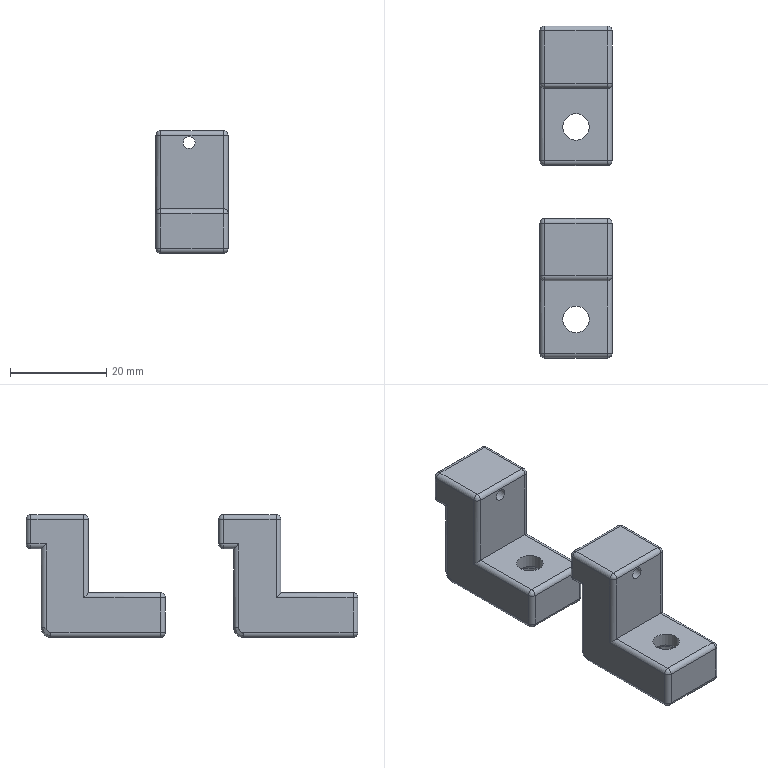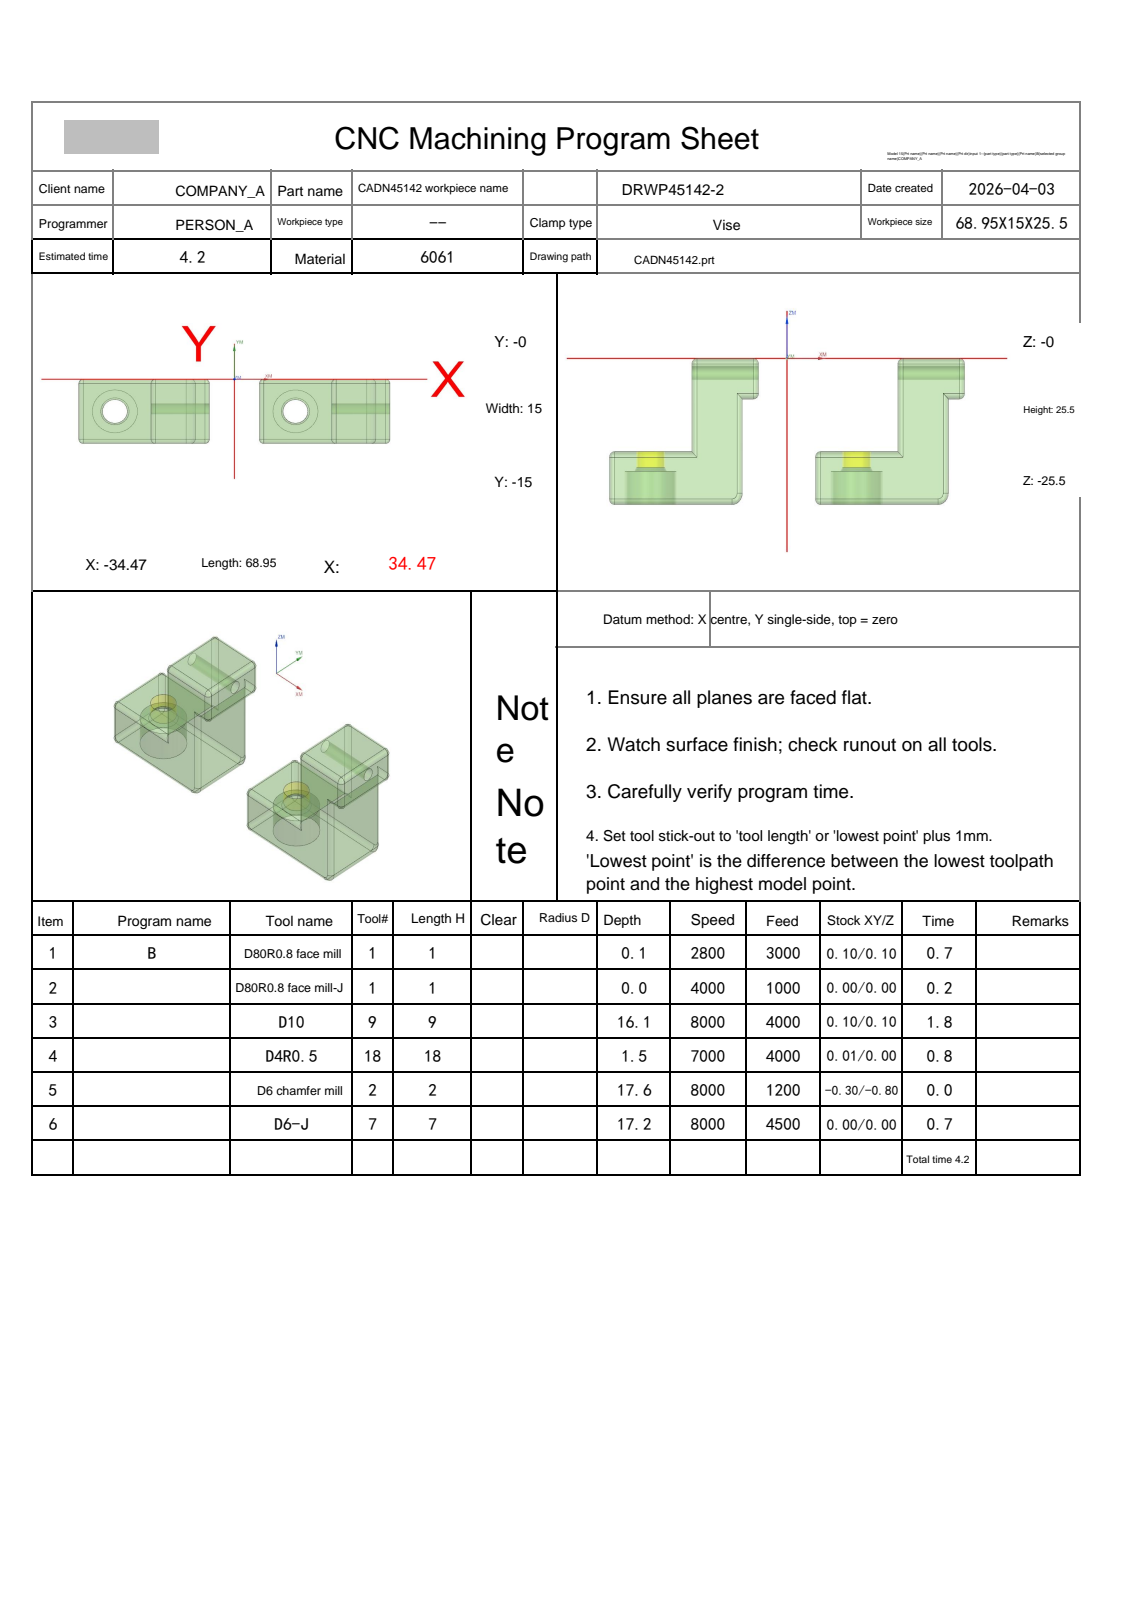NC program | NX | posted by the shop | part box 15 x 68.95 x 25.5 mm
Lines 1498 to 2892 of 8513:
N4 T18 M06
(D4R0.5  D=4. R=0.5 H=18 ce=0.01 di=0.00)
G00 G90 G54 X20.847 Y-13.574 M03 S7000
G43 H18 Z20.
M08
Z1.5
G01 Y-.87 Z.834 F4000.
X20.907 Y-.536 Z.816
X21.034 Y-.22 Z.799
X21.221 Y.064 Z.781
X21.461 Y.304 Z.763
X21.745 Y.491 Z.745
X22.061 Y.618 Z.727
X22.396 Y.678 Z.71
X33.604 Z.122
X33.939 Y.618 Z.104
X34.255 Y.491 Z.086
X34.539 Y.304 Z.069
X34.779 Y.064 Z.051
X34.966 Y-.22 Z.033
X35.093 Y-.536 Z.015
X35.153 Y-.87 Z-.003
Y-1. Z-.009
Y-14.
G02 X33.475 Y-15.678 I-1.678 J0.0
G01 X22.525
G02 X20.847 Y-14. I0.0 J1.678
G01 Y-1.
G02 X22.525 Y.678 I1.678 J0.0
G01 X33.475
G02 X35.153 Y-1. I0.0 J-1.678
G01 X35.155 Y-2.625 Z-.01
X35.16 Y-4.25
X35.163 Y-5.875 Z-.011
X35.167 Y-7.5
X35.17 Y-9.125 Z-.012
X35.175 Y-10.75
X35.177 Y-12.375 Z-.013
X35.181 Y-14.
X35.177 Y-14.122
X35.164 Y-14.243
X35.143 Y-14.363
X35.113 Y-14.481
X35.075 Y-14.597
X35.028 Y-14.709
X34.974 Y-14.818
X34.912 Y-14.923
X34.843 Y-15.024
X34.766 Y-15.119
X34.683 Y-15.208
X34.594 Y-15.291
X34.499 Y-15.368
X34.399 Y-15.438
X34.294 Y-15.501
X34.185 Y-15.555
X34.073 Y-15.602 Z-.014
X33.957 Y-15.641
X33.838 Y-15.672
X33.718 Y-15.693
X33.597 Y-15.707
X33.475 Y-15.711
X31.65 Y-15.714
X29.825 Y-15.718 Z-.015
X28. Y-15.721
X26.175 Y-15.725 Z-.016
X24.35 Y-15.728
X22.525 Y-15.732 Z-.017
X22.402 Y-15.728
X22.279 Y-15.715
X22.157 Y-15.693
X22.037 Y-15.663
X21.919 Y-15.624
X21.805 Y-15.577
X21.694 Y-15.522
X21.588 Y-15.459
X21.486 Y-15.388
X21.389 Y-15.311
X21.298 Y-15.226
X21.214 Y-15.136
X21.136 Y-15.04
X21.065 Y-14.938
X21.002 Y-14.832
X20.946 Y-14.721
X20.899 Y-14.606
X20.859 Y-14.489
X20.828 Y-14.369
X20.806 Y-14.247
X20.793 Y-14.124
X20.788 Y-14.
X20.785 Y-12.375 Z-.018
X20.783 Y-10.75
X20.78 Y-9.125 Z-.019
X20.777 Y-7.5
X20.774 Y-5.875 Z-.02
X20.772 Y-4.25
X20.769 Y-2.625
X20.766 Y-1. Z-.021
X20.77 Y-.874
X20.784 Y-.75
X20.806 Y-.626
X20.837 Y-.504
X20.876 Y-.385
X20.924 Y-.269
X20.98 Y-.156
X21.044 Y-.048
X21.116 Y.055
X21.194 Y.153
X21.28 Y.245
X21.372 Y.331
X21.47 Y.41
X21.573 Y.482
X21.681 Y.547
X21.793 Y.603
X21.909 Y.651
X22.029 Y.691
X22.151 Y.723 Z-.022
X22.274 Y.745
X22.399 Y.759
X22.525 Y.764
X24.35 Y.765
X26.175 Y.769 Z-.023
X28. Y.771
X29.825 Y.774 Z-.024
X31.65 Y.777
X33.475 Y.78 Z-.025
X33.602 Y.776
X33.728 Y.762
X33.853 Y.74
X33.976 Y.708
X34.097 Y.669
X34.215 Y.62
X34.328 Y.563
X34.438 Y.499
X34.543 Y.426
X34.642 Y.347
X34.735 Y.26
X34.822 Y.167
X34.902 Y.068
X34.974 Y-.036
X35.04 Y-.146
X35.097 Y-.259
X35.146 Y-.377
X35.186 Y-.498
X35.218 Y-.621
X35.24 Y-.746
X35.254 Y-.873
X35.259 Y-1.
X35.262 Y-2.625 Z-.026
X35.265 Y-4.25 Z-.027
X35.268 Y-5.875
X35.272 Y-7.5 Z-.028
X35.275 Y-9.125
X35.278 Y-10.75 Z-.029
X35.281 Y-12.375 Z-.03
X35.284 Y-14.
X35.28 Y-14.129
X35.266 Y-14.257
X35.243 Y-14.385
X35.212 Y-14.51
X35.171 Y-14.632
X35.122 Y-14.752 Z-.031
X35.064 Y-14.868
X34.998 Y-14.979
X34.925 Y-15.085
X34.844 Y-15.186
X34.756 Y-15.281
X34.661 Y-15.369
X34.561 Y-15.451
X34.455 Y-15.525
X34.344 Y-15.591
X34.228 Y-15.649
X34.108 Y-15.699
X33.986 Y-15.74
X33.86 Y-15.772
X33.733 Y-15.795
X33.604 Y-15.809
X33.475 Y-15.814
X31.65 Y-15.817 Z-.032
X29.825 Y-15.821 Z-.033
X28. Y-15.824
X26.175 Y-15.827 Z-.034
X24.35 Y-15.83 Z-.035
X22.525 Y-15.834
X22.394 Y-15.829
X22.264 Y-15.816 Z-.036
X22.135 Y-15.792
X22.008 Y-15.76
X21.884 Y-15.719
X21.763 Y-15.669
X21.646 Y-15.611
X21.533 Y-15.544
X21.425 Y-15.469
X21.323 Y-15.387
X21.227 Y-15.298
X21.137 Y-15.202
X21.055 Y-15.1
X20.98 Y-14.993
X20.913 Y-14.88
X20.854 Y-14.763
X20.804 Y-14.642
X20.762 Y-14.518
X20.729 Y-14.39
X20.706 Y-14.261
X20.691 Y-14.131
X20.686 Y-14. Z-.037
X20.684 Y-12.375
X20.681 Y-10.75 Z-.038
X20.679 Y-9.125
X20.676 Y-7.5 Z-.039
X20.674 Y-5.875 Z-.04
X20.671 Y-4.25
X20.668 Y-2.625 Z-.041
X20.665 Y-1.
X20.67 Y-.867
X20.684 Y-.735 Z-.042
X20.707 Y-.605
X20.74 Y-.476
X20.782 Y-.35
X20.832 Y-.227
X20.892 Y-.108
X20.959 Y.006
X21.035 Y.116
X21.118 Y.219
X21.209 Y.317
X21.306 Y.407
X21.409 Y.491
X21.518 Y.567
X21.632 Y.635
X21.751 Y.695
X21.874 Y.746
X22. Y.788
X22.129 Y.821
X22.26 Y.845
X22.392 Y.859
X22.525 Y.865 Z-.043
X24.35 Y.867
X26.175 Y.87 Z-.044
X28. Y.872 Z-.045
X29.825 Y.875
X31.65 Y.878 Z-.046
X33.475 Y.881 Z-.047
X33.609 Y.876
X33.742 Y.862
X33.875 Y.839
X34.005 Y.805
X34.132 Y.763
X34.257 Y.712
X34.377 Y.652
X34.492 Y.584
X34.603 Y.507
X34.708 Y.423
X34.806 Y.332
X34.898 Y.233
X34.983 Y.129
X35.059 Y.018
X35.128 Y-.097
X35.188 Y-.217
X35.24 Y-.342 Z-.048
X35.283 Y-.469
X35.316 Y-.599
X35.34 Y-.732
X35.355 Y-.866
X35.36 Y-1.
X35.363 Y-2.625 Z-.049
X35.366 Y-4.25
X35.369 Y-5.875 Z-.05
X35.372 Y-7.5 Z-.051
X35.375 Y-9.125 Z-.052
X35.378 Y-10.75
X35.38 Y-12.375 Z-.053
X35.383 Y-14. Z-.054
X35.382 Y-14.068
X35.379 Y-14.136
X35.373 Y-14.204
X35.364 Y-14.271
X35.354 Y-14.339
X35.34 Y-14.406
X35.325 Y-14.472
X35.307 Y-14.538
X35.287 Y-14.603
X35.264 Y-14.667
X35.239 Y-14.731
X35.212 Y-14.793
X35.183 Y-14.855
X35.151 Y-14.915
X35.118 Y-14.975
X35.082 Y-15.033 Z-.055
X35.044 Y-15.09
X35.004 Y-15.145
X34.963 Y-15.199
X34.919 Y-15.251
X34.874 Y-15.302
X34.826 Y-15.351
X34.777 Y-15.399
X34.726 Y-15.444
X34.674 Y-15.488
X34.62 Y-15.53
X34.565 Y-15.57
X34.508 Y-15.608
X34.45 Y-15.644
X34.391 Y-15.678
X34.331 Y-15.71
X34.269 Y-15.739
X34.207 Y-15.767
X34.143 Y-15.792
X34.079 Y-15.815
X34.014 Y-15.835
X33.948 Y-15.853
X33.881 Y-15.869
X33.814 Y-15.883
X33.747 Y-15.894
X33.679 Y-15.902
X33.611 Y-15.908
X33.543 Y-15.912
X33.475 Y-15.913
X31.65 Y-15.917 Z-.056
X29.825 Y-15.92 Z-.057
X28. Y-15.923 Z-.058
X26.175 Y-15.926 Z-.059
X24.35 Y-15.929 Z-.06
X22.525 Y-15.932 Z-.061
X22.456 Y-15.931
X22.387 Y-15.927
X22.319 Y-15.921
X22.25 Y-15.913
X22.182 Y-15.902
X22.114 Y-15.889
X22.047 Y-15.873
X21.981 Y-15.855
X21.915 Y-15.834
X21.85 Y-15.811
X21.785 Y-15.786
X21.722 Y-15.759
X21.66 Y-15.729
X21.598 Y-15.697
X21.538 Y-15.663
X21.48 Y-15.627
X21.422 Y-15.589
X21.366 Y-15.548
X21.311 Y-15.506
X21.258 Y-15.462
X21.207 Y-15.416
X21.157 Y-15.368
X21.109 Y-15.318
X21.063 Y-15.267
X21.018 Y-15.214 Z-.062
X20.976 Y-15.16
X20.936 Y-15.104
X20.897 Y-15.046
X20.861 Y-14.987
X20.826 Y-14.927
X20.794 Y-14.866
X20.764 Y-14.804
X20.737 Y-14.741
X20.711 Y-14.676
X20.688 Y-14.611
X20.667 Y-14.545
X20.649 Y-14.479
X20.633 Y-14.411
X20.619 Y-14.344
X20.608 Y-14.275
X20.599 Y-14.207
X20.593 Y-14.138
X20.589 Y-14.069
X20.588 Y-14.
X20.586 Y-12.375 Z-.063
X20.583 Y-10.75 Z-.064
X20.581 Y-9.125
X20.578 Y-7.5 Z-.065
X20.575 Y-5.875 Z-.066
X20.573 Y-4.25 Z-.067
X20.57 Y-2.625 Z-.068
X20.568 Y-1.
X20.569 Y-.93
X20.572 Y-.86
X20.578 Y-.791
X20.587 Y-.721 Z-.069
X20.598 Y-.652
X20.612 Y-.584
X20.628 Y-.516
X20.646 Y-.448
X20.667 Y-.381
X20.69 Y-.316
X20.715 Y-.25
X20.743 Y-.186
X20.773 Y-.123
X20.806 Y-.061
X20.84 Y0.0
X20.877 Y.059
X20.916 Y.118
X20.957 Y.174
X20.999 Y.23
X21.044 Y.283
X21.091 Y.336
X21.139 Y.386
X21.19 Y.435
X21.242 Y.481
X21.295 Y.526
X21.35 Y.569
X21.407 Y.61
X21.465 Y.649
X21.525 Y.686
X21.586 Y.721
X21.647 Y.754
X21.711 Y.784
X21.775 Y.812
X21.84 Y.838 Z-.07
X21.906 Y.861
X21.973 Y.882
X22.04 Y.901
X22.108 Y.917
X22.177 Y.931
X22.246 Y.942
X22.316 Y.951
X22.385 Y.957
X22.455 Y.961
X22.525 Y.962
X24.35 Y.965 Z-.071
X26.175 Y.968 Z-.072
X28. Y.97
X29.825 Y.973 Z-.073
X31.65 Y.976 Z-.074
X33.475 Y.978 Z-.075
X33.545
X33.616 Y.974
X33.686 Y.968
X33.756 Y.959
X33.826 Y.948
X33.895 Y.934
X33.964 Y.918
X34.032 Y.899
X34.1 Y.878
X34.167 Y.855
X34.232 Y.829
X34.297 Y.801 Z-.076
X34.361 Y.771
X34.424 Y.738
X34.485 Y.703
X34.545 Y.666
X34.604 Y.627
X34.662 Y.585
X34.718 Y.542
X34.772 Y.497
X34.825 Y.45
X34.875 Y.401
X34.925 Y.35
X34.972 Y.297
X35.017 Y.243
X35.061 Y.187
X35.102 Y.13
X35.142 Y.071
X35.179 Y.011
X35.214 Y-.05
X35.247 Y-.113
X35.277 Y-.177
X35.306 Y-.241
X35.332 Y-.307
X35.356 Y-.374
X35.377 Y-.442
X35.396 Y-.51
X35.412 Y-.579
X35.426 Y-.648
X35.437 Y-.718
X35.446 Y-.788 Z-.077
X35.452 Y-.859
X35.457 Y-.929
X35.458 Y-1.
X35.46 Y-2.625 Z-.078
X35.463 Y-4.25
X35.466 Y-5.875 Z-.079
X35.469 Y-7.5 Z-.08
X35.471 Y-9.125 Z-.081
X35.475 Y-10.75 Z-.082
X35.477 Y-12.375 Z-.083
X35.48 Y-14. Z-.084
X35.476 Y-14.131
X35.463 Y-14.262
X35.442 Y-14.391
X35.412 Y-14.519
X35.375 Y-14.645 Z-.085
X35.328 Y-14.768
X35.275 Y-14.887
X35.213 Y-15.003
X35.144 Y-15.115
X35.067 Y-15.222
X34.984 Y-15.323
X34.894 Y-15.419
X34.799 Y-15.509
X34.697 Y-15.593
X34.591 Y-15.67
X34.479 Y-15.739
X34.363 Y-15.801
X34.244 Y-15.856 Z-.086
X34.121 Y-15.902
X33.995 Y-15.941
X33.867 Y-15.971
X33.737 Y-15.992
X33.606 Y-16.006
X33.475 Y-16.01
X31.65 Y-16.013 Z-.087
X29.825 Y-16.016 Z-.088
X28. Y-16.019 Z-.089
X26.175 Y-16.022 Z-.09
X24.35 Y-16.024 Z-.091
X22.525 Y-16.028 Z-.092
X22.393 Y-16.024
X22.26 Y-16.011
X22.129 Y-15.989 Z-.093
X22. Y-15.959
X21.873 Y-15.921
X21.749 Y-15.875
X21.628 Y-15.82
X21.51 Y-15.758
X21.398 Y-15.687
X21.289 Y-15.61
X21.187 Y-15.526
X21.089 Y-15.436
X20.999 Y-15.339
X20.914 Y-15.236
X20.836 Y-15.128
X20.766 Y-15.015 Z-.094
X20.703 Y-14.898
X20.648 Y-14.777
X20.601 Y-14.653
X20.562 Y-14.526
X20.532 Y-14.396
X20.51 Y-14.265
X20.497 Y-14.133
X20.492 Y-14.
X20.49 Y-12.375 Z-.095
X20.487 Y-10.75 Z-.096
X20.485 Y-9.125 Z-.097
X20.482 Y-7.5 Z-.098
X20.48 Y-5.875 Z-.099
X20.477 Y-4.25 Z-.1
X20.475 Y-2.625 Z-.101
X20.473 Y-1. Z-.102
X20.477 Y-.866
X20.49 Y-.732
X20.511 Y-.599
X20.542 Y-.469
X20.58 Y-.34
X20.628 Y-.214
X20.683 Y-.091
X20.746 Y.027
X20.817 Y.141
X20.895 Y.251
X20.98 Y.355 Z-.103
X21.072 Y.453
X21.17 Y.545
X21.274 Y.631
X21.383 Y.709
X21.497 Y.78
X21.616 Y.844
X21.738 Y.9
X21.864 Y.947
X21.993 Y.987
X22.124 Y1.017
X22.257 Y1.04
X22.391 Y1.053
X22.525 Y1.058 Z-.104
X24.35 Y1.06 Z-.105
X26.175 Y1.063 Z-.106
X28. Y1.065 Z-.107
X29.825 Y1.068 Z-.108
X31.65 Y1.071 Z-.109
X33.475 Y1.073 Z-.11
X33.61 Y1.069
X33.745 Y1.056
X33.879 Y1.034
X34.012 Y1.003
X34.142 Y.964
X34.269 Y.917
X34.392 Y.861
X34.512 Y.797 Z-.111
X34.628 Y.725
X34.738 Y.646
X34.843 Y.56
X34.942 Y.468
X35.036 Y.369
X35.122 Y.264
X35.201 Y.154
X35.273 Y.038
X35.337 Y-.082
X35.393 Y-.205
X35.442 Y-.332
X35.481 Y-.462
X35.512 Y-.595 Z-.112
X35.535 Y-.729
X35.548 Y-.864
X35.553 Y-1.
X35.555 Y-2.625 Z-.113
X35.558 Y-4.25 Z-.114
X35.561 Y-5.875 Z-.115
X35.563 Y-7.5 Z-.116
X35.566 Y-9.125 Z-.117
X35.569 Y-10.75 Z-.118
X35.571 Y-12.375 Z-.119
X35.574 Y-14. Z-.121
X35.57 Y-14.137
X35.556 Y-14.274
X35.534 Y-14.409
X35.503 Y-14.543
X35.463 Y-14.675
X35.415 Y-14.804
X35.359 Y-14.929
X35.294 Y-15.05
X35.222 Y-15.167
X35.142 Y-15.279
X35.055 Y-15.385 Z-.122
X34.961 Y-15.486
X34.861 Y-15.58
X34.754 Y-15.667
X34.643 Y-15.748
X34.526 Y-15.821
X34.405 Y-15.886
X34.279 Y-15.943
X34.151 Y-15.991
X34.019 Y-16.031
X33.885 Y-16.063 Z-.123
X33.749 Y-16.085
X33.612 Y-16.099
X33.475 Y-16.104
X31.65 Y-16.107 Z-.124
X29.825 Y-16.11 Z-.125
X28. Y-16.113 Z-.126
X26.175 Y-16.115 Z-.128
X24.35 Y-16.118 Z-.129
X22.525 Y-16.121 Z-.13
X22.386 Y-16.116
X22.248 Y-16.103
X22.111 Y-16.081
X21.976 Y-16.049 Z-.131
X21.843 Y-16.009
X21.713 Y-15.961
X21.586 Y-15.903
X21.464 Y-15.838
X21.346 Y-15.765
X21.233 Y-15.684
X21.125 Y-15.596
X21.024 Y-15.501
X20.929 Y-15.4
X20.84 Y-15.293
X20.759 Y-15.18 Z-.132
X20.685 Y-15.062
X20.62 Y-14.939
X20.562 Y-14.813
X20.513 Y-14.683
X20.472 Y-14.55
X20.441 Y-14.414
X20.418 Y-14.277
X20.404 Y-14.139
X20.399 Y-14.
X20.397 Y-12.375 Z-.134
X20.394 Y-10.75 Z-.135
X20.392 Y-9.125 Z-.136
X20.39 Y-7.5 Z-.137
X20.387 Y-5.875 Z-.138
X20.385 Y-4.25 Z-.139
X20.383 Y-2.625 Z-.14
X20.38 Y-1. Z-.141
X20.385 Y-.86
X20.398 Y-.72
X20.421 Y-.581
X20.452 Y-.445 Z-.142
X20.493 Y-.31
X20.542 Y-.179
X20.6 Y-.051
X20.666 Y.073
X20.74 Y.193
X20.822 Y.307
X20.911 Y.416
X21.007 Y.519
X21.109 Y.615
X21.218 Y.704
X21.332 Y.786 Z-.143
X21.451 Y.861
X21.575 Y.927
X21.703 Y.985
X21.834 Y1.035
X21.969 Y1.076
X22.106 Y1.108
X22.245 Y1.131
X22.385 Y1.145
X22.525 Y1.15
X24.35 Y1.152 Z-.145
X26.175 Y1.155 Z-.146
X28. Y1.158 Z-.147
X29.825 Y1.16 Z-.148
X31.65 Y1.163 Z-.15
X33.475 Y1.165 Z-.151
X33.616 Y1.161
X33.757 Y1.147
X33.897 Y1.124
X34.035 Y1.092
X34.171 Y1.051
X34.304 Y1.002
X34.433 Y.943
X34.558 Y.877 Z-.152
X34.679 Y.802
X34.794 Y.719
X34.904 Y.63
X35.008 Y.533
X35.105 Y.429
X35.195 Y.32
X35.278 Y.205
X35.353 Y.084
X35.42 Y-.041
X35.479 Y-.17 Z-.153
X35.529 Y-.303
X35.57 Y-.439
X35.603 Y-.577
X35.626 Y-.717
X35.64 Y-.858
X35.645 Y-1.
X35.647 Y-2.625 Z-.154
X35.65 Y-4.25 Z-.156
X35.652 Y-5.875 Z-.157
X35.655 Y-7.5 Z-.158
X35.657 Y-9.125 Z-.159
X35.66 Y-10.75 Z-.161
X35.662 Y-12.375 Z-.162
X35.665 Y-14. Z-.163
X35.66 Y-14.143
X35.646 Y-14.286
X35.623 Y-14.427
X35.591 Y-14.567
X35.55 Y-14.704 Z-.164
X35.499 Y-14.838
X35.44 Y-14.969
X35.373 Y-15.096
X35.297 Y-15.218
X35.214 Y-15.334
X35.123 Y-15.445
X35.025 Y-15.55
X34.921 Y-15.648
X34.81 Y-15.74 Z-.165
X34.693 Y-15.823
X34.571 Y-15.899
X34.445 Y-15.967
X34.314 Y-16.027
X34.18 Y-16.077
X34.043 Y-16.119
X33.903 Y-16.152
X33.761 Y-16.176
X33.618 Y-16.19 Z-.166
X33.475 Y-16.195
X31.65 Y-16.197 Z-.167
X29.825 Y-16.2 Z-.168
X28. Y-16.203 Z-.17
X26.175 Y-16.206 Z-.171
X24.35 Y-16.208 Z-.173
X22.525 Y-16.211 Z-.174
X22.381 Y-16.206
X22.237 Y-16.193
X22.094 Y-16.169
X21.953 Y-16.136 Z-.175
X21.814 Y-16.095
X21.679 Y-16.044
X21.547 Y-15.984
X21.419 Y-15.916
X21.296 Y-15.84
X21.178 Y-15.756
X21.066 Y-15.664
X20.96 Y-15.565
X20.861 Y-15.459 Z-.176
X20.769 Y-15.348
X20.684 Y-15.23
X20.607 Y-15.107
X20.539 Y-14.979
X20.479 Y-14.847
X20.428 Y-14.712
X20.385 Y-14.573
X20.352 Y-14.432
X20.328 Y-14.289
X20.314 Y-14.145 Z-.177
X20.309 Y-14.
X20.307 Y-12.375 Z-.178
X20.304 Y-10.75 Z-.179
X20.302 Y-9.125 Z-.18
X20.3 Y-7.5 Z-.182
X20.298 Y-5.875 Z-.183
X20.295 Y-4.25 Z-.184
X20.293 Y-2.625 Z-.185
X20.291 Y-1. Z-.187
X20.295 Y-.854
X20.309 Y-.708
X20.333 Y-.564
X20.366 Y-.421
X20.408 Y-.281
X20.46 Y-.144
X20.52 Y-.011
X20.589 Y.118 Z-.188
X20.666 Y.242
X20.751 Y.362
X20.844 Y.475
X20.944 Y.582
X21.05 Y.682
X21.163 Y.775
X21.282 Y.86
X21.406 Y.938
X21.535 Y1.007 Z-.189
X21.669 Y1.068
X21.806 Y1.12
X21.946 Y1.162
X22.089 Y1.196
X22.233 Y1.22
X22.379 Y1.234
X22.525 Y1.239
X24.35 Y1.242 Z-.191
X26.175 Y1.244 Z-.192
X28. Y1.247 Z-.194
X29.825 Y1.249 Z-.195
X31.65 Y1.252 Z-.196
X33.475 Y1.254 Z-.198
X33.622 Y1.25
X33.769 Y1.235
X33.915 Y1.211
X34.058 Y1.178
X34.2 Y1.135
X34.338 Y1.084
X34.472 Y1.023 Z-.199
X34.603 Y.954
X34.728 Y.876
X34.848 Y.79
X34.962 Y.696
X35.07 Y.596
X35.171 Y.488
X35.265 Y.374
X35.352 Y.254
X35.43 Y.129 Z-.2
X35.499 Y-.002
X35.561 Y-.136
X35.613 Y-.274
X35.656 Y-.416
X35.69 Y-.559
X35.714 Y-.705
X35.729 Y-.852
X35.734 Y-1.
X35.736 Y-2.625 Z-.202
X35.738 Y-4.25 Z-.203
X35.741 Y-5.875 Z-.205
X35.743 Y-7.5 Z-.206
X35.746 Y-9.125 Z-.207
X35.748 Y-10.75 Z-.209
X35.75 Y-12.375 Z-.21
X35.753 Y-14. Z-.211
X35.752 Y-14.074 Z-.212
X35.748 Y-14.149
X35.742 Y-14.223
X35.733 Y-14.297
X35.723 Y-14.371
X35.709 Y-14.444
X35.694 Y-14.517
X35.676 Y-14.589
X35.655 Y-14.661
X35.633 Y-14.732
X35.608 Y-14.803
X35.58 Y-14.872
X35.551 Y-14.94
X35.519 Y-15.008
X35.485 Y-15.074
X35.449 Y-15.139
X35.411 Y-15.204 Z-.213
X35.37 Y-15.266
X35.328 Y-15.328
X35.284 Y-15.388
X35.237 Y-15.446
X35.189 Y-15.503
X35.139 Y-15.559
X35.087 Y-15.612
X35.034 Y-15.664
X34.978 Y-15.714
X34.922 Y-15.763
X34.863 Y-15.809
X34.803 Y-15.854
X34.742 Y-15.896
X34.679 Y-15.937
X34.615 Y-15.975 Z-.214
X34.55 Y-16.012
X34.484 Y-16.046
X34.416 Y-16.078
X34.348 Y-16.108
X34.279 Y-16.135
X34.208 Y-16.16
X34.137 Y-16.183
X34.065 Y-16.204
X33.993 Y-16.222
X33.92 Y-16.238
X33.847 Y-16.252
X33.773 Y-16.263
X33.698 Y-16.271
X33.624 Y-16.277
X33.549 Y-16.281
X33.475 Y-16.283 Z-.215
X31.65 Y-16.285 Z-.216
X29.825 Y-16.288 Z-.218
X28. Y-16.29 Z-.219
X26.175 Y-16.293 Z-.221
X24.35 Y-16.295 Z-.222
X22.525 Y-16.298 Z-.224
X22.45 Y-16.297
X22.375 Y-16.293
X22.3 Y-16.287
X22.225 Y-16.279
X22.151 Y-16.268
X22.077 Y-16.254
X22.003 Y-16.239
X21.93 Y-16.22
X21.858 Y-16.2
X21.786 Y-16.177
X21.715 Y-16.152 Z-.225
X21.645 Y-16.124
X21.576 Y-16.094
X21.508 Y-16.062
X21.441 Y-16.028
X21.375 Y-15.992
X21.311 Y-15.953
X21.247 Y-15.912
X21.185 Y-15.869
X21.125 Y-15.825
X21.066 Y-15.778
X21.008 Y-15.729
X20.953 Y-15.679
X20.898 Y-15.627
X20.846 Y-15.573
X20.795 Y-15.517
X20.747 Y-15.459 Z-.226
X20.7 Y-15.401
X20.655 Y-15.34
X20.612 Y-15.278
X20.571 Y-15.215
X20.532 Y-15.151
X20.495 Y-15.085
X20.461 Y-15.018
X20.429 Y-14.95
X20.398 Y-14.881
X20.371 Y-14.811
X20.345 Y-14.74
X20.322 Y-14.668
X20.301 Y-14.596
X20.283 Y-14.523
X20.267 Y-14.449 Z-.227
X20.253 Y-14.375
X20.242 Y-14.3
X20.233 Y-14.225
X20.227 Y-14.15
X20.223 Y-14.075
X20.222 Y-14.
X20.22 Y-12.375 Z-.228
X20.218 Y-10.75 Z-.23
X20.216 Y-9.125 Z-.231
X20.213 Y-7.5 Z-.232
X20.211 Y-5.875 Z-.234
X20.209 Y-4.25 Z-.235
X20.207 Y-2.625 Z-.237
X20.205 Y-1. Z-.238
X20.206 Y-.924
X20.21 Y-.848
X20.215 Y-.773
X20.224 Y-.697
X20.235 Y-.622
X20.249 Y-.547
X20.265 Y-.473
X20.283 Y-.399
X20.304 Y-.326 Z-.239
X20.327 Y-.254
X20.352 Y-.182
X20.38 Y-.112
X20.41 Y-.042
X20.443 Y.027
X20.477 Y.095
X20.514 Y.161
X20.553 Y.226
X20.594 Y.29
X20.637 Y.353
X20.683 Y.414
X20.73 Y.474
X20.779 Y.531
X20.83 Y.588
X20.883 Y.643 Z-.24
X20.937 Y.696
X20.993 Y.747
X21.051 Y.796
X21.111 Y.843
X21.172 Y.889
X21.234 Y.932
X21.298 Y.973
X21.363 Y1.012
X21.43 Y1.05
X21.497 Y1.084
X21.566 Y1.117
X21.636 Y1.147
X21.706 Y1.175
X21.778 Y1.201
X21.85 Y1.224
X21.924 Y1.245 Z-.241
X21.997 Y1.264
X22.072 Y1.28
X22.147 Y1.294
X22.222 Y1.305
X22.297 Y1.314
X22.373 Y1.32
X22.449 Y1.324
X22.525 Y1.325
X24.35 Y1.328 Z-.243
X26.175 Y1.33 Z-.244
X28. Y1.332 Z-.246
X29.825 Y1.335 Z-.247
X31.65 Y1.337 Z-.249
X33.475 Y1.34 Z-.25
X33.551 Y1.338
X33.628 Y1.335
X33.704 Y1.329 Z-.251
X33.78 Y1.32
X33.856 Y1.309
X33.931 Y1.295
X34.006 Y1.279
X34.08 Y1.261
X34.154 Y1.24
X34.227 Y1.216
X34.299 Y1.191
X34.371 Y1.163
X34.441 Y1.132
X34.51 Y1.099
X34.578 Y1.065
X34.645 Y1.027
X34.711 Y.988
X34.776 Y.947 Z-.252
X34.839 Y.903
X34.9 Y.858
X34.96 Y.81
X35.019 Y.761
X35.076 Y.709
X35.131 Y.656
X35.184 Y.601
X35.236 Y.544
X35.285 Y.486
X35.333 Y.426
X35.379 Y.364
X35.422 Y.301
X35.464 Y.237
X35.504 Y.171
X35.541 Y.104 Z-.253
X35.576 Y.036
X35.609 Y-.033
X35.639 Y-.103
X35.668 Y-.175
X35.694 Y-.247
X35.717 Y-.32
X35.738 Y-.393
X35.757 Y-.468
X35.773 Y-.543
X35.787 Y-.618
X35.799 Y-.694
X35.808 Y-.77
X35.814 Y-.847
X35.818 Y-.923
X35.819 Y-1.
X35.821 Y-2.625 Z-.255
X35.824 Y-4.25 Z-.257
X35.826 Y-5.875 Z-.258
X35.828 Y-7.5 Z-.26
X35.83 Y-9.125 Z-.261
X35.832 Y-10.75 Z-.263
X35.835 Y-12.375 Z-.264
X35.837 Y-14. Z-.266
X35.833 Y-14.142
X35.82 Y-14.285
X35.799 Y-14.426
X35.769 Y-14.565
X35.731 Y-14.703
X35.684 Y-14.838
X35.63 Y-14.97 Z-.267
X35.568 Y-15.098
X35.498 Y-15.223
X35.42 Y-15.343
X35.336 Y-15.458
X35.244 Y-15.568
X35.147 Y-15.672
X35.043 Y-15.77
X34.933 Y-15.861 Z-.268
X34.818 Y-15.946
X34.698 Y-16.024
X34.574 Y-16.094
X34.446 Y-16.157
X34.314 Y-16.212
X34.179 Y-16.259
X34.041 Y-16.297 Z-.269
X33.901 Y-16.327
X33.76 Y-16.349
X33.618 Y-16.362
X33.475 Y-16.367
X31.65 Y-16.369 Z-.271
X29.825 Y-16.372 Z-.272
X28. Y-16.374 Z-.274
X26.175 Y-16.376 Z-.276
X24.35 Y-16.379 Z-.278
X22.525 Y-16.381 Z-.279
X22.381 Y-16.377
X22.238 Y-16.364 Z-.28
X22.096 Y-16.343
X21.955 Y-16.313
X21.816 Y-16.274
X21.68 Y-16.228
X21.547 Y-16.173
X21.418 Y-16.11
X21.292 Y-16.039
X21.171 Y-15.961 Z-.281
X21.055 Y-15.876
X20.944 Y-15.784
X20.84 Y-15.685
X20.741 Y-15.581
X20.648 Y-15.47
X20.563 Y-15.354
X20.484 Y-15.233 Z-.282
X20.413 Y-15.108
X20.35 Y-14.979
X20.295 Y-14.846
X20.248 Y-14.709
X20.209 Y-14.571
X20.179 Y-14.43
X20.157 Y-14.287
X20.143 Y-14.144 Z-.283
X20.139 Y-14.
X20.137 Y-12.375 Z-.284
X20.135 Y-10.75 Z-.286
X20.133 Y-9.125 Z-.287
X20.131 Y-7.5 Z-.289
X20.129 Y-5.875 Z-.29
X20.126 Y-4.25 Z-.292
X20.124 Y-2.625 Z-.293
X20.122 Y-1. Z-.295
X20.127 Y-.855
X20.14 Y-.71
X20.161 Y-.567
X20.191 Y-.425
X20.23 Y-.285 Z-.296
X20.277 Y-.148
X20.333 Y-.013
X20.396 Y.117
X20.467 Y.244
X20.546 Y.366
X20.632 Y.483
X20.725 Y.595
X20.824 Y.701 Z-.297
X20.93 Y.801
X21.042 Y.894
X21.159 Y.98
X21.281 Y1.059
X21.407 Y1.131
X21.538 Y1.194
X21.672 Y1.25 Z-.298
X21.809 Y1.298
X21.949 Y1.337
X22.091 Y1.368
X22.235 Y1.39
X22.38 Y1.403
X22.525 Y1.408
X24.35 Y1.41 Z-.3
X26.175 Y1.412 Z-.302
X28. Y1.414 Z-.303
X29.825 Y1.417 Z-.305
X31.65 Y1.419 Z-.307
X33.475 Y1.421 Z-.309
X33.621 Y1.417
X33.767 Y1.404
X33.911 Y1.382
X34.054 Y1.351
X34.195 Y1.312
X34.334 Y1.265
X34.469 Y1.209
X34.601 Y1.145 Z-.31
X34.728 Y1.073
X34.851 Y.994
X34.969 Y.907
X35.082 Y.814
X35.188 Y.714
X35.289 Y.607
X35.383 Y.495 Z-.311
X35.47 Y.377
X35.549 Y.254
X35.621 Y.127
X35.686 Y-.005
X35.742 Y-.14
X35.79 Y-.279
X35.829 Y-.42 Z-.312
X35.86 Y-.563
X35.882 Y-.708
X35.896 Y-.854
X35.901 Y-1.
X35.903 Y-2.625 Z-.314
X35.905 Y-4.25 Z-.315
X35.907 Y-5.875 Z-.317
X35.909 Y-7.5 Z-.319
X35.911 Y-9.125 Z-.32
X35.913 Y-10.75 Z-.322
X35.915 Y-12.375 Z-.324
X35.917 Y-14. Z-.325
X35.913 Y-14.147
X35.9 Y-14.294
X35.878 Y-14.44 Z-.326
X35.847 Y-14.584
X35.808 Y-14.727
X35.76 Y-14.866
X35.703 Y-15.003
X35.639 Y-15.136
X35.566 Y-15.264 Z-.327
X35.486 Y-15.388
X35.399 Y-15.507
X35.305 Y-15.621
X35.204 Y-15.729
X35.096 Y-15.83
X34.983 Y-15.925
X34.864 Y-16.012 Z-.328
X34.74 Y-16.093
X34.611 Y-16.165
X34.479 Y-16.23
X34.342 Y-16.287
X34.203 Y-16.335
X34.06 Y-16.375
X33.916 Y-16.406 Z-.329
X33.77 Y-16.429
X33.622 Y-16.442
X33.475 Y-16.447
X31.65 Y-16.449 Z-.331
X29.825 Y-16.452 Z-.333
X28. Y-16.454 Z-.335
X26.175 Y-16.456 Z-.336
X24.35 Y-16.458 Z-.338
X22.525 Y-16.461 Z-.34
X22.377 Y-16.456
X22.229 Y-16.443
X22.082 Y-16.421 Z-.341
X21.936 Y-16.39
X21.793 Y-16.35
X21.652 Y-16.302
X21.515 Y-16.245
X21.381 Y-16.18
X21.251 Y-16.107
X21.126 Y-16.027 Z-.342
X21.006 Y-15.939
X20.892 Y-15.844
X20.783 Y-15.742
X20.681 Y-15.633
X20.586 Y-15.519
X20.497 Y-15.399
X20.417 Y-15.274 Z-.343
X20.343 Y-15.145
X20.278 Y-15.011
X20.221 Y-14.874
X20.172 Y-14.733
X20.132 Y-14.59
X20.1 Y-14.444 Z-.344
X20.078 Y-14.297
X20.064 Y-14.149
X20.059 Y-14.
X20.058 Y-12.375 Z-.346
X20.056 Y-10.75 Z-.347
X20.054 Y-9.125 Z-.349
X20.052 Y-7.5 Z-.351
X20.05 Y-5.875 Z-.352
X20.048 Y-4.25 Z-.354
X20.046 Y-2.625 Z-.355
X20.044 Y-1. Z-.357
X20.048 Y-.85
X20.062 Y-.701
X20.084 Y-.553
X20.115 Y-.406 Z-.358
X20.155 Y-.262
X20.204 Y-.12
X20.261 Y.019
X20.327 Y.154
X20.4 Y.284
X20.482 Y.411 Z-.359
X20.57 Y.531
X20.666 Y.647
X20.769 Y.756
X20.878 Y.859
X20.993 Y.955
X21.114 Y1.044
X21.24 Y1.126 Z-.36
X21.371 Y1.2
X21.506 Y1.266
X21.644 Y1.323
X21.786 Y1.372
X21.931 Y1.413
X22.077 Y1.445 Z-.361
X22.226 Y1.467
X22.375 Y1.481
X22.525 Y1.486
X24.35 Y1.488 Z-.363
X26.175 Y1.49 Z-.365
X28. Y1.492 Z-.366
X29.825 Y1.495 Z-.368
X31.65 Y1.497 Z-.37
X33.475 Y1.499 Z-.372
X33.626 Y1.494
X33.776 Y1.481
X33.925 Y1.458
X34.073 Y1.427 Z-.373
X34.218 Y1.386
X34.361 Y1.337
X34.501 Y1.28
X34.637 Y1.214
X34.768 Y1.14
X34.895 Y1.058 Z-.374
X35.017 Y.968
X35.133 Y.872
X35.243 Y.768
X35.347 Y.658
X35.444 Y.543
X35.533 Y.421
X35.616 Y.294 Z-.375
X35.69 Y.163
X35.756 Y.027
X35.814 Y-.113
X35.864 Y-.256
X35.904 Y-.401
X35.936 Y-.549
X35.959 Y-.698 Z-.376
X35.973 Y-.849
X35.978 Y-1.
X35.98 Y-2.625 Z-.378
X35.982 Y-4.25 Z-.379
X35.984 Y-5.875 Z-.381
X35.986 Y-7.5 Z-.383
X35.988 Y-9.125 Z-.385
X35.99 Y-10.75 Z-.386
X35.992 Y-12.375 Z-.388
X35.993 Y-14. Z-.39
X35.989 Y-14.152
X35.975 Y-14.303
X35.953 Y-14.454
X35.921 Y-14.603 Z-.391
X35.88 Y-14.749
X35.831 Y-14.893
X35.773 Y-15.034
X35.706 Y-15.171
X35.632 Y-15.304
X35.549 Y-15.432 Z-.392
X35.459 Y-15.554
X35.362 Y-15.671
X35.257 Y-15.782
X35.147 Y-15.887
X35.03 Y-15.985
X34.907 Y-16.075 Z-.393
X34.779 Y-16.158
X34.647 Y-16.233
X34.51 Y-16.3
X34.369 Y-16.358
X34.225 Y-16.408
X34.078 Y-16.449 Z-.394
X33.93 Y-16.481
X33.779 Y-16.504
X33.627 Y-16.518
X33.475 Y-16.523
X31.65 Y-16.525 Z-.396
X29.825 Y-16.527 Z-.398
X28. Y-16.529 Z-.4
X26.175 Y-16.532 Z-.402
X24.35 Y-16.534 Z-.404
X22.525 Y-16.536 Z-.406
X22.372 Y-16.531
X22.219 Y-16.518
X22.068 Y-16.495 Z-.407
X21.918 Y-16.463
X21.77 Y-16.422
X21.626 Y-16.372
X21.484 Y-16.314
X21.346 Y-16.247
X21.212 Y-16.171 Z-.408
X21.083 Y-16.088
X20.96 Y-15.998
X20.842 Y-15.9
X20.73 Y-15.795
X20.625 Y-15.683
X20.527 Y-15.565
X20.436 Y-15.442 Z-.409
X20.352 Y-15.313
X20.277 Y-15.18
X20.21 Y-15.042
X20.151 Y-14.9
X20.1 Y-14.755
X20.059 Y-14.608 Z-.41
X20.027 Y-14.458
X20.003 Y-14.306
X19.989 Y-14.153
X19.984 Y-14.
X19.983 Y-12.375 Z-.412
X19.981 Y-10.75 Z-.414
X19.979 Y-9.125 Z-.416
X19.977 Y-7.5 Z-.417
X19.975 Y-5.875 Z-.419
X19.974 Y-4.25 Z-.421